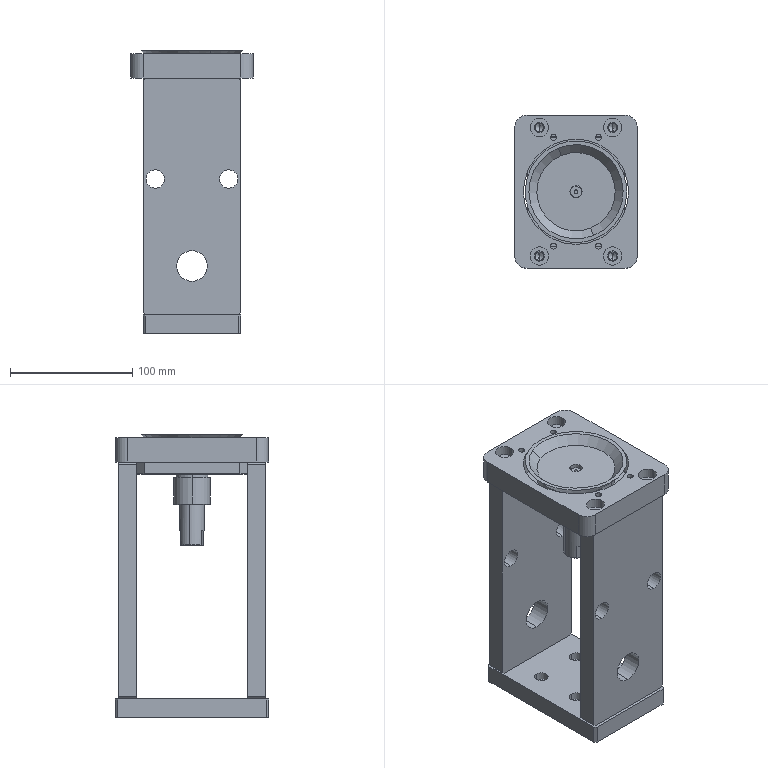Part | SolidWorks | 7 solids | 252 faces | box 100 x 125 x 230.841 mm | volume 827561 mm3 | cylinder 128 | plane 79 | cone 45 | commonest cylinder face diameters 15 x24 6.6 x16 6.8 x16 8.5 x10 5 x8 9 x8